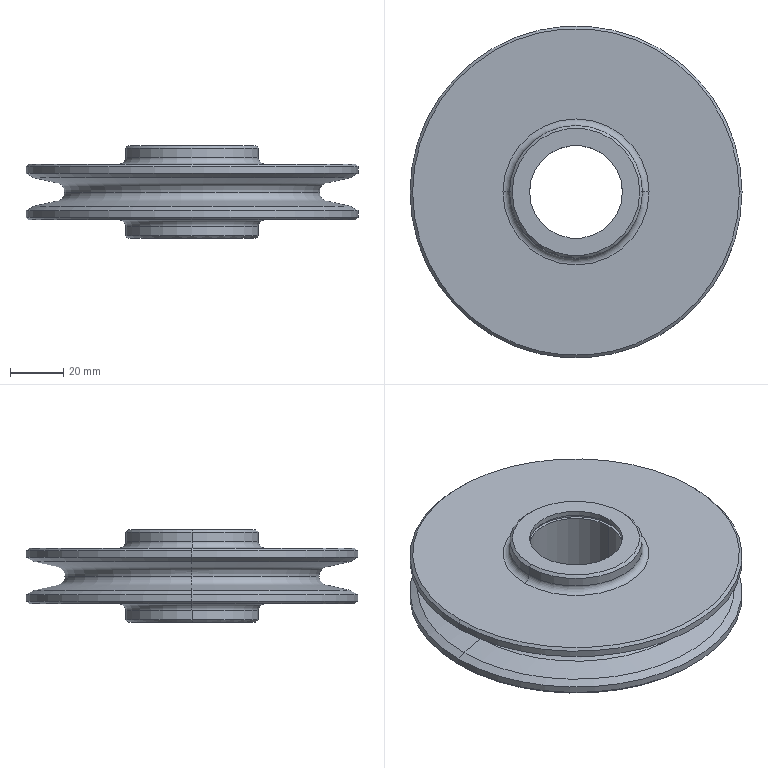Part | STEP file | POLEA IZAJE_MAMELON | 1 solid | 50 faces | box 125 x 125 x 35 mm | volume 205749 mm3 | cylinder 18 | cone 16 | torus 8 | plane 8 | commonest cylinder face diameters 35 x6 37.2 x4 50 x4 125 x4
STEP:
#1=CARTESIAN_POINT('',(-50.742,0.,-3.417));
#2=VERTEX_POINT('',#1);
#3=CARTESIAN_POINT('',(-48.,0.,0.));
#4=VERTEX_POINT('',#3);
#5=CARTESIAN_POINT('',(-51.5,0.,0.));
#6=DIRECTION('',(0.,-1.,0.));
#7=DIRECTION('',(0.,0.,-1.));
#8=AXIS2_PLACEMENT_3D('',#5,#6,#7);
#9=CIRCLE('',#8,3.5);
#10=EDGE_CURVE('',#2,#4,#9,.T.);
#11=ORIENTED_EDGE('',*,*,#10,.T.);
#12=CARTESIAN_POINT('',(48.,0.,0.));
#13=VERTEX_POINT('',#12);
#14=CARTESIAN_POINT('',(0.,0.,0.));
#15=DIRECTION('',(0.,0.,-1.));
#16=DIRECTION('',(-1.,0.,0.));
#17=AXIS2_PLACEMENT_3D('',#14,#15,#16);
#18=CIRCLE('',#17,48.);
#19=EDGE_CURVE('',#4,#13,#18,.T.);
#20=ORIENTED_EDGE('',*,*,#19,.T.);
#21=CARTESIAN_POINT('',(50.742,0.,-3.417));
#22=VERTEX_POINT('',#21);
#23=CARTESIAN_POINT('',(51.5,0.,0.));
#24=DIRECTION('',(0.,1.,0.));
#25=DIRECTION('',(-1.,0.,0.));
#26=AXIS2_PLACEMENT_3D('',#23,#24,#25);
#27=CIRCLE('',#26,3.5);
#28=EDGE_CURVE('',#22,#13,#27,.T.);
#29=ORIENTED_EDGE('',*,*,#28,.F.);
#30=CARTESIAN_POINT('',(0.,0.,-3.417));
#31=DIRECTION('',(0.,0.,-1.));
#32=DIRECTION('',(-1.,0.,0.));
#33=AXIS2_PLACEMENT_3D('',#30,#31,#32);
#34=CIRCLE('',#33,50.742);
#35=EDGE_CURVE('',#2,#22,#34,.T.);
#36=ORIENTED_EDGE('',*,*,#35,.F.);
#37=EDGE_LOOP('',(#11,#20,#29,#36));
#38=FACE_OUTER_BOUND('',#37,.T.);
#39=CARTESIAN_POINT('',(0.,0.,0.));
#40=DIRECTION('',(0.,0.,-1.));
#41=DIRECTION('',(-1.,0.,0.));
#42=AXIS2_PLACEMENT_3D('',#39,#40,#41);
#43=TOROIDAL_SURFACE('',#42,51.5,3.5);
#44=ADVANCED_FACE('',(#38),#43,.F.);
#45=ORIENTED_EDGE('',*,*,#28,.T.);
#46=CARTESIAN_POINT('',(0.,0.,0.));
#47=DIRECTION('',(0.,0.,-1.));
#48=DIRECTION('',(-1.,0.,0.));
#49=AXIS2_PLACEMENT_3D('',#46,#47,#48);
#50=CIRCLE('',#49,48.);
#51=EDGE_CURVE('',#13,#4,#50,.T.);
#52=ORIENTED_EDGE('',*,*,#51,.T.);
#53=ORIENTED_EDGE('',*,*,#10,.F.);
#54=CARTESIAN_POINT('',(0.,0.,-3.417));
#55=DIRECTION('',(0.,0.,-1.));
#56=DIRECTION('',(-1.,0.,0.));
#57=AXIS2_PLACEMENT_3D('',#54,#55,#56);
#58=CIRCLE('',#57,50.742);
#59=EDGE_CURVE('',#22,#2,#58,.T.);
#60=ORIENTED_EDGE('',*,*,#59,.F.);
#61=EDGE_LOOP('',(#45,#52,#53,#60));
#62=FACE_OUTER_BOUND('',#61,.T.);
#63=CARTESIAN_POINT('',(0.,0.,0.));
#64=DIRECTION('',(0.,0.,-1.));
#65=DIRECTION('',(-1.,0.,0.));
#66=AXIS2_PLACEMENT_3D('',#63,#64,#65);
#67=TOROIDAL_SURFACE('',#66,51.5,3.5);
#68=ADVANCED_FACE('',(#62),#67,.F.);
#69=CARTESIAN_POINT('',(61.5,0.,10.5));
#70=VERTEX_POINT('',#69);
#71=CARTESIAN_POINT('',(-61.5,0.,10.5));
#72=VERTEX_POINT('',#71);
#73=CARTESIAN_POINT('',(0.,0.,10.5));
#74=DIRECTION('',(0.,0.,1.));
#75=DIRECTION('',(-1.,0.,0.));
#76=AXIS2_PLACEMENT_3D('',#73,#74,#75);
#77=CIRCLE('',#76,61.5);
#78=EDGE_CURVE('',#70,#72,#77,.T.);
#79=ORIENTED_EDGE('',*,*,#78,.F.);
#80=CARTESIAN_POINT('',(62.5,0.,9.5));
#81=VERTEX_POINT('',#80);
#82=CARTESIAN_POINT('',(62.5,0.,9.5));
#83=DIRECTION('',(0.7071,0.,-0.7071));
#84=VECTOR('',#83,1000.);
#85=LINE('',#82,#84);
#86=EDGE_CURVE('',#70,#81,#85,.T.);
#87=ORIENTED_EDGE('',*,*,#86,.T.);
#88=CARTESIAN_POINT('',(-62.5,0.,9.5));
#89=VERTEX_POINT('',#88);
#90=CARTESIAN_POINT('',(0.,0.,9.5));
#91=DIRECTION('',(0.,0.,-1.));
#92=DIRECTION('',(-1.,0.,0.));
#93=AXIS2_PLACEMENT_3D('',#90,#91,#92);
#94=CIRCLE('',#93,62.5);
#95=EDGE_CURVE('',#89,#81,#94,.T.);
#96=ORIENTED_EDGE('',*,*,#95,.F.);
#97=CARTESIAN_POINT('',(-62.5,0.,9.5));
#98=DIRECTION('',(-0.7071,0.,-0.7071));
#99=VECTOR('',#98,1000.);
#100=LINE('',#97,#99);
#101=EDGE_CURVE('',#72,#89,#100,.T.);
#102=ORIENTED_EDGE('',*,*,#101,.F.);
#103=EDGE_LOOP('',(#79,#87,#96,#102));
#104=FACE_OUTER_BOUND('',#103,.T.);
#105=CARTESIAN_POINT('',(0.,0.,9.5));
#106=DIRECTION('',(0.,0.,-1.));
#107=DIRECTION('',(-1.,0.,0.));
#108=AXIS2_PLACEMENT_3D('',#105,#106,#107);
#109=CONICAL_SURFACE('',#108,62.5,0.7854);
#110=ADVANCED_FACE('',(#104),#109,.T.);
#111=CARTESIAN_POINT('',(-61.5,0.,-10.5));
#112=VERTEX_POINT('',#111);
#113=CARTESIAN_POINT('',(61.5,0.,-10.5));
#114=VERTEX_POINT('',#113);
#115=CARTESIAN_POINT('',(0.,0.,-10.5));
#116=DIRECTION('',(0.,0.,-1.));
#117=DIRECTION('',(1.,0.,0.));
#118=AXIS2_PLACEMENT_3D('',#115,#116,#117);
#119=CIRCLE('',#118,61.5);
#120=EDGE_CURVE('',#112,#114,#119,.T.);
#121=ORIENTED_EDGE('',*,*,#120,.F.);
#122=CARTESIAN_POINT('',(-62.5,0.,-9.5));
#123=VERTEX_POINT('',#122);
#124=CARTESIAN_POINT('',(-62.5,0.,-9.5));
#125=DIRECTION('',(-0.7071,0.,0.7071));
#126=VECTOR('',#125,1000.);
#127=LINE('',#124,#126);
#128=EDGE_CURVE('',#112,#123,#127,.T.);
#129=ORIENTED_EDGE('',*,*,#128,.T.);
#130=CARTESIAN_POINT('',(62.5,0.,-9.5));
#131=VERTEX_POINT('',#130);
#132=CARTESIAN_POINT('',(0.,0.,-9.5));
#133=DIRECTION('',(0.,0.,1.));
#134=DIRECTION('',(1.,0.,0.));
#135=AXIS2_PLACEMENT_3D('',#132,#133,#134);
#136=CIRCLE('',#135,62.5);
#137=EDGE_CURVE('',#131,#123,#136,.T.);
#138=ORIENTED_EDGE('',*,*,#137,.F.);
#139=CARTESIAN_POINT('',(62.5,0.,-9.5));
#140=DIRECTION('',(0.7071,0.,0.7071));
#141=VECTOR('',#140,1000.);
#142=LINE('',#139,#141);
#143=EDGE_CURVE('',#114,#131,#142,.T.);
#144=ORIENTED_EDGE('',*,*,#143,.F.);
#145=EDGE_LOOP('',(#121,#129,#138,#144));
#146=FACE_OUTER_BOUND('',#145,.T.);
#147=CARTESIAN_POINT('',(0.,0.,-9.5));
#148=DIRECTION('',(0.,0.,1.));
#149=DIRECTION('',(1.,0.,0.));
#150=AXIS2_PLACEMENT_3D('',#147,#148,#149);
#151=CONICAL_SURFACE('',#150,62.5,0.7854);
#152=ADVANCED_FACE('',(#146),#151,.T.);
#153=CARTESIAN_POINT('',(18.6,0.,15.6));
#154=VERTEX_POINT('',#153);
#155=CARTESIAN_POINT('',(-18.6,0.,15.6));
#156=VERTEX_POINT('',#155);
#157=CARTESIAN_POINT('',(0.,0.,15.6));
#158=DIRECTION('',(0.,0.,-1.));
#159=DIRECTION('',(-1.,0.,0.));
#160=AXIS2_PLACEMENT_3D('',#157,#158,#159);
#161=CIRCLE('',#160,18.6);
#162=EDGE_CURVE('',#154,#156,#161,.T.);
#163=ORIENTED_EDGE('',*,*,#162,.F.);
#164=CARTESIAN_POINT('',(18.6,0.,14.2));
#165=VERTEX_POINT('',#164);
#166=CARTESIAN_POINT('',(18.6,0.,-24.658));
#167=DIRECTION('',(0.,0.,-1.));
#168=VECTOR('',#167,1000.);
#169=LINE('',#166,#168);
#170=EDGE_CURVE('',#154,#165,#169,.T.);
#171=ORIENTED_EDGE('',*,*,#170,.T.);
#172=CARTESIAN_POINT('',(-18.6,0.,14.2));
#173=VERTEX_POINT('',#172);
#174=CARTESIAN_POINT('',(0.,0.,14.2));
#175=DIRECTION('',(0.,0.,-1.));
#176=DIRECTION('',(-1.,0.,0.));
#177=AXIS2_PLACEMENT_3D('',#174,#175,#176);
#178=CIRCLE('',#177,18.6);
#179=EDGE_CURVE('',#165,#173,#178,.T.);
#180=ORIENTED_EDGE('',*,*,#179,.T.);
#181=CARTESIAN_POINT('',(-18.6,0.,-24.658));
#182=DIRECTION('',(0.,0.,-1.));
#183=VECTOR('',#182,1000.);
#184=LINE('',#181,#183);
#185=EDGE_CURVE('',#156,#173,#184,.T.);
#186=ORIENTED_EDGE('',*,*,#185,.F.);
#187=EDGE_LOOP('',(#163,#171,#180,#186));
#188=FACE_OUTER_BOUND('',#187,.T.);
#189=CARTESIAN_POINT('',(0.,0.,-24.658));
#190=DIRECTION('',(0.,0.,-1.));
#191=DIRECTION('',(-1.,0.,0.));
#192=AXIS2_PLACEMENT_3D('',#189,#190,#191);
#193=CYLINDRICAL_SURFACE('',#192,18.6);
#194=ADVANCED_FACE('',(#188),#193,.F.);
#195=CARTESIAN_POINT('',(-17.5,0.,-14.2));
#196=VERTEX_POINT('',#195);
#197=CARTESIAN_POINT('',(17.5,0.,-14.2));
#198=VERTEX_POINT('',#197);
#199=CARTESIAN_POINT('',(0.,0.,-14.2));
#200=DIRECTION('',(0.,0.,1.));
#201=DIRECTION('',(-1.,0.,0.));
#202=AXIS2_PLACEMENT_3D('',#199,#200,#201);
#203=CIRCLE('',#202,17.5);
#204=EDGE_CURVE('',#196,#198,#203,.T.);
#205=ORIENTED_EDGE('',*,*,#204,.F.);
#206=CARTESIAN_POINT('',(-17.5,0.,14.2));
#207=VERTEX_POINT('',#206);
#208=CARTESIAN_POINT('',(-17.5,0.,-17.5));
#209=DIRECTION('',(0.,0.,1.));
#210=VECTOR('',#209,1000.);
#211=LINE('',#208,#210);
#212=EDGE_CURVE('',#196,#207,#211,.T.);
#213=ORIENTED_EDGE('',*,*,#212,.T.);
#214=CARTESIAN_POINT('',(17.5,0.,14.2));
#215=VERTEX_POINT('',#214);
#216=CARTESIAN_POINT('',(0.,0.,14.2));
#217=DIRECTION('',(0.,0.,-1.));
#218=DIRECTION('',(1.,0.,0.));
#219=AXIS2_PLACEMENT_3D('',#216,#217,#218);
#220=CIRCLE('',#219,17.5);
#221=EDGE_CURVE('',#215,#207,#220,.T.);
#222=ORIENTED_EDGE('',*,*,#221,.F.);
#223=CARTESIAN_POINT('',(17.5,0.,-17.5));
#224=DIRECTION('',(0.,0.,1.));
#225=VECTOR('',#224,1000.);
#226=LINE('',#223,#225);
#227=EDGE_CURVE('',#198,#215,#226,.T.);
#228=ORIENTED_EDGE('',*,*,#227,.F.);
#229=EDGE_LOOP('',(#205,#213,#222,#228));
#230=FACE_OUTER_BOUND('',#229,.T.);
#231=CARTESIAN_POINT('',(0.,0.,-17.5));
#232=DIRECTION('',(0.,0.,1.));
#233=DIRECTION('',(1.,0.,0.));
#234=AXIS2_PLACEMENT_3D('',#231,#232,#233);
#235=CYLINDRICAL_SURFACE('',#234,17.5);
#236=ADVANCED_FACE('',(#230),#235,.F.);
#237=CARTESIAN_POINT('',(18.6,0.,-14.2));
#238=VERTEX_POINT('',#237);
#239=CARTESIAN_POINT('',(-18.6,0.,-14.2));
#240=VERTEX_POINT('',#239);
#241=CARTESIAN_POINT('',(0.,0.,-14.2));
#242=DIRECTION('',(0.,0.,-1.));
#243=DIRECTION('',(-1.,0.,0.));
#244=AXIS2_PLACEMENT_3D('',#241,#242,#243);
#245=CIRCLE('',#244,18.6);
#246=EDGE_CURVE('',#238,#240,#245,.T.);
#247=ORIENTED_EDGE('',*,*,#246,.F.);
#248=CARTESIAN_POINT('',(18.6,0.,-15.6));
#249=VERTEX_POINT('',#248);
#250=CARTESIAN_POINT('',(18.6,0.,-24.658));
#251=DIRECTION('',(0.,0.,-1.));
#252=VECTOR('',#251,1000.);
#253=LINE('',#250,#252);
#254=EDGE_CURVE('',#238,#249,#253,.T.);
#255=ORIENTED_EDGE('',*,*,#254,.T.);
#256=CARTESIAN_POINT('',(-18.6,0.,-15.6));
#257=VERTEX_POINT('',#256);
#258=CARTESIAN_POINT('',(0.,0.,-15.6));
#259=DIRECTION('',(0.,0.,-1.));
#260=DIRECTION('',(-1.,0.,0.));
#261=AXIS2_PLACEMENT_3D('',#258,#259,#260);
#262=CIRCLE('',#261,18.6);
#263=EDGE_CURVE('',#249,#257,#262,.T.);
#264=ORIENTED_EDGE('',*,*,#263,.T.);
#265=CARTESIAN_POINT('',(-18.6,0.,-24.658));
#266=DIRECTION('',(0.,0.,-1.));
#267=VECTOR('',#266,1000.);
#268=LINE('',#265,#267);
#269=EDGE_CURVE('',#240,#257,#268,.T.);
#270=ORIENTED_EDGE('',*,*,#269,.F.);
#271=EDGE_LOOP('',(#247,#255,#264,#270));
#272=FACE_OUTER_BOUND('',#271,.T.);
#273=CARTESIAN_POINT('',(0.,0.,-24.658));
#274=DIRECTION('',(0.,0.,-1.));
#275=DIRECTION('',(-1.,0.,0.));
#276=AXIS2_PLACEMENT_3D('',#273,#274,#275);
#277=CYLINDRICAL_SURFACE('',#276,18.6);
#278=ADVANCED_FACE('',(#272),#277,.F.);
#279=CARTESIAN_POINT('',(24.,0.,17.5));
#280=VERTEX_POINT('',#279);
#281=CARTESIAN_POINT('',(-24.,0.,17.5));
#282=VERTEX_POINT('',#281);
#283=CARTESIAN_POINT('',(0.,0.,17.5));
#284=DIRECTION('',(0.,0.,1.));
#285=DIRECTION('',(-1.,0.,0.));
#286=AXIS2_PLACEMENT_3D('',#283,#284,#285);
#287=CIRCLE('',#286,24.);
#288=EDGE_CURVE('',#280,#282,#287,.T.);
#289=ORIENTED_EDGE('',*,*,#288,.F.);
#290=CARTESIAN_POINT('',(25.,0.,16.5));
#291=VERTEX_POINT('',#290);
#292=CARTESIAN_POINT('',(25.,0.,16.5));
#293=DIRECTION('',(0.7071,0.,-0.7071));
#294=VECTOR('',#293,1000.);
#295=LINE('',#292,#294);
#296=EDGE_CURVE('',#280,#291,#295,.T.);
#297=ORIENTED_EDGE('',*,*,#296,.T.);
#298=CARTESIAN_POINT('',(-25.,0.,16.5));
#299=VERTEX_POINT('',#298);
#300=CARTESIAN_POINT('',(0.,0.,16.5));
#301=DIRECTION('',(0.,0.,-1.));
#302=DIRECTION('',(-1.,0.,0.));
#303=AXIS2_PLACEMENT_3D('',#300,#301,#302);
#304=CIRCLE('',#303,25.);
#305=EDGE_CURVE('',#299,#291,#304,.T.);
#306=ORIENTED_EDGE('',*,*,#305,.F.);
#307=CARTESIAN_POINT('',(-25.,0.,16.5));
#308=DIRECTION('',(-0.7071,0.,-0.7071));
#309=VECTOR('',#308,1000.);
#310=LINE('',#307,#309);
#311=EDGE_CURVE('',#282,#299,#310,.T.);
#312=ORIENTED_EDGE('',*,*,#311,.F.);
#313=EDGE_LOOP('',(#289,#297,#306,#312));
#314=FACE_OUTER_BOUND('',#313,.T.);
#315=CARTESIAN_POINT('',(0.,0.,16.5));
#316=DIRECTION('',(0.,0.,-1.));
#317=DIRECTION('',(-1.,0.,0.));
#318=AXIS2_PLACEMENT_3D('',#315,#316,#317);
#319=CONICAL_SURFACE('',#318,25.,0.7854);
#320=ADVANCED_FACE('',(#314),#319,.T.);
#321=CARTESIAN_POINT('',(-24.,0.,-17.5));
#322=VERTEX_POINT('',#321);
#323=CARTESIAN_POINT('',(24.,0.,-17.5));
#324=VERTEX_POINT('',#323);
#325=CARTESIAN_POINT('',(0.,0.,-17.5));
#326=DIRECTION('',(0.,0.,-1.));
#327=DIRECTION('',(1.,0.,0.));
#328=AXIS2_PLACEMENT_3D('',#325,#326,#327);
#329=CIRCLE('',#328,24.);
#330=EDGE_CURVE('',#322,#324,#329,.T.);
#331=ORIENTED_EDGE('',*,*,#330,.F.);
#332=CARTESIAN_POINT('',(-25.,0.,-16.5));
#333=VERTEX_POINT('',#332);
#334=CARTESIAN_POINT('',(-24.,0.,-17.5));
#335=DIRECTION('',(-0.7071,0.,0.7071));
#336=VECTOR('',#335,1000.);
#337=LINE('',#334,#336);
#338=EDGE_CURVE('',#322,#333,#337,.T.);
#339=ORIENTED_EDGE('',*,*,#338,.T.);
#340=CARTESIAN_POINT('',(25.,0.,-16.5));
#341=VERTEX_POINT('',#340);
#342=CARTESIAN_POINT('',(0.,0.,-16.5));
#343=DIRECTION('',(0.,0.,1.));
#344=DIRECTION('',(1.,0.,0.));
#345=AXIS2_PLACEMENT_3D('',#342,#343,#344);
#346=CIRCLE('',#345,25.);
#347=EDGE_CURVE('',#341,#333,#346,.T.);
#348=ORIENTED_EDGE('',*,*,#347,.F.);
#349=CARTESIAN_POINT('',(24.,0.,-17.5));
#350=DIRECTION('',(0.7071,0.,0.7071));
#351=VECTOR('',#350,1000.);
#352=LINE('',#349,#351);
#353=EDGE_CURVE('',#324,#341,#352,.T.);
#354=ORIENTED_EDGE('',*,*,#353,.F.);
#355=EDGE_LOOP('',(#331,#339,#348,#354));
#356=FACE_OUTER_BOUND('',#355,.T.);
#357=CARTESIAN_POINT('',(0.,0.,-17.5));
#358=DIRECTION('',(0.,0.,1.));
#359=DIRECTION('',(1.,0.,0.));
#360=AXIS2_PLACEMENT_3D('',#357,#358,#359);
#361=CONICAL_SURFACE('',#360,24.,0.7854);
#362=ADVANCED_FACE('',(#356),#361,.T.);
#363=CARTESIAN_POINT('',(-59.688,0.,5.4));
#364=VERTEX_POINT('',#363);
#365=CARTESIAN_POINT('',(59.688,0.,5.4));
#366=VERTEX_POINT('',#365);
#367=CARTESIAN_POINT('',(0.,0.,5.4));
#368=DIRECTION('',(0.,0.,-1.));
#369=DIRECTION('',(-1.,0.,0.));
#370=AXIS2_PLACEMENT_3D('',#367,#368,#369);
#371=CIRCLE('',#370,59.688);
#372=EDGE_CURVE('',#364,#366,#371,.T.);
#373=ORIENTED_EDGE('',*,*,#372,.F.);
#374=CARTESIAN_POINT('',(-62.5,0.,7.024));
#375=VERTEX_POINT('',#374);
#376=CARTESIAN_POINT('',(-59.688,0.,5.4));
#377=DIRECTION('',(-0.866,0.,0.5));
#378=VECTOR('',#377,1000.);
#379=LINE('',#376,#378);
#380=EDGE_CURVE('',#364,#375,#379,.T.);
#381=ORIENTED_EDGE('',*,*,#380,.T.);
#382=CARTESIAN_POINT('',(62.5,0.,7.024));
#383=VERTEX_POINT('',#382);
#384=CARTESIAN_POINT('',(0.,0.,7.024));
#385=DIRECTION('',(0.,0.,1.));
#386=DIRECTION('',(1.,0.,0.));
#387=AXIS2_PLACEMENT_3D('',#384,#385,#386);
#388=CIRCLE('',#387,62.5);
#389=EDGE_CURVE('',#383,#375,#388,.T.);
#390=ORIENTED_EDGE('',*,*,#389,.F.);
#391=CARTESIAN_POINT('',(59.688,0.,5.4));
#392=DIRECTION('',(0.866,0.,0.5));
#393=VECTOR('',#392,1000.);
#394=LINE('',#391,#393);
#395=EDGE_CURVE('',#366,#383,#394,.T.);
#396=ORIENTED_EDGE('',*,*,#395,.F.);
#397=EDGE_LOOP('',(#373,#381,#390,#396));
#398=FACE_OUTER_BOUND('',#397,.T.);
#399=CARTESIAN_POINT('',(0.,0.,5.4));
#400=DIRECTION('',(0.,0.,1.));
#401=DIRECTION('',(1.,0.,0.));
#402=AXIS2_PLACEMENT_3D('',#399,#400,#401);
#403=CONICAL_SURFACE('',#402,59.688,1.047);
#404=ADVANCED_FACE('',(#398),#403,.T.);
#405=CARTESIAN_POINT('',(59.688,0.,-5.4));
#406=VERTEX_POINT('',#405);
#407=CARTESIAN_POINT('',(-59.688,0.,-5.4));
#408=VERTEX_POINT('',#407);
#409=CARTESIAN_POINT('',(0.,0.,-5.4));
#410=DIRECTION('',(0.,0.,1.));
#411=DIRECTION('',(1.,0.,0.));
#412=AXIS2_PLACEMENT_3D('',#409,#410,#411);
#413=CIRCLE('',#412,59.688);
#414=EDGE_CURVE('',#406,#408,#413,.T.);
#415=ORIENTED_EDGE('',*,*,#414,.F.);
#416=CARTESIAN_POINT('',(62.5,0.,-7.024));
#417=VERTEX_POINT('',#416);
#418=CARTESIAN_POINT('',(62.5,0.,-7.024));
#419=DIRECTION('',(0.866,0.,-0.5));
#420=VECTOR('',#419,1000.);
#421=LINE('',#418,#420);
#422=EDGE_CURVE('',#406,#417,#421,.T.);
#423=ORIENTED_EDGE('',*,*,#422,.T.);
#424=CARTESIAN_POINT('',(-62.5,0.,-7.024));
#425=VERTEX_POINT('',#424);
#426=CARTESIAN_POINT('',(0.,0.,-7.024));
#427=DIRECTION('',(0.,0.,-1.));
#428=DIRECTION('',(-1.,0.,0.));
#429=AXIS2_PLACEMENT_3D('',#426,#427,#428);
#430=CIRCLE('',#429,62.5);
#431=EDGE_CURVE('',#425,#417,#430,.T.);
#432=ORIENTED_EDGE('',*,*,#431,.F.);
#433=CARTESIAN_POINT('',(-62.5,0.,-7.024));
#434=DIRECTION('',(-0.866,0.,-0.5));
#435=VECTOR('',#434,1000.);
#436=LINE('',#433,#435);
#437=EDGE_CURVE('',#408,#425,#436,.T.);
#438=ORIENTED_EDGE('',*,*,#437,.F.);
#439=EDGE_LOOP('',(#415,#423,#432,#438));
#440=FACE_OUTER_BOUND('',#439,.T.);
#441=CARTESIAN_POINT('',(0.,0.,-7.024));
#442=DIRECTION('',(0.,0.,-1.));
#443=DIRECTION('',(-1.,0.,0.));
#444=AXIS2_PLACEMENT_3D('',#441,#442,#443);
#445=CONICAL_SURFACE('',#444,62.5,1.047);
#446=ADVANCED_FACE('',(#440),#445,.T.);
#447=CARTESIAN_POINT('',(27.5,0.,10.5));
#448=VERTEX_POINT('',#447);
#449=CARTESIAN_POINT('',(-27.5,0.,10.5));
#450=VERTEX_POINT('',#449);
#451=CARTESIAN_POINT('',(0.,0.,10.5));
#452=DIRECTION('',(0.,0.,-1.));
#453=DIRECTION('',(-1.,0.,0.));
#454=AXIS2_PLACEMENT_3D('',#451,#452,#453);
#455=CIRCLE('',#454,27.5);
#456=EDGE_CURVE('',#448,#450,#455,.T.);
#457=ORIENTED_EDGE('',*,*,#456,.F.);
#458=CARTESIAN_POINT('',(25.,0.,13.));
#459=VERTEX_POINT('',#458);
#460=CARTESIAN_POINT('',(27.5,0.,13.));
#461=DIRECTION('',(0.,1.,0.));
#462=DIRECTION('',(-1.,0.,0.));
#463=AXIS2_PLACEMENT_3D('',#460,#461,#462);
#464=CIRCLE('',#463,2.5);
#465=EDGE_CURVE('',#448,#459,#464,.T.);
#466=ORIENTED_EDGE('',*,*,#465,.T.);
#467=CARTESIAN_POINT('',(-25.,0.,13.));
#468=VERTEX_POINT('',#467);
#469=CARTESIAN_POINT('',(0.,0.,13.));
#470=DIRECTION('',(0.,0.,1.));
#471=DIRECTION('',(-1.,0.,0.));
#472=AXIS2_PLACEMENT_3D('',#469,#470,#471);
#473=CIRCLE('',#472,25.);
#474=EDGE_CURVE('',#468,#459,#473,.T.);
#475=ORIENTED_EDGE('',*,*,#474,.F.);
#476=CARTESIAN_POINT('',(-27.5,0.,13.));
#477=DIRECTION('',(0.,-1.,0.));
#478=DIRECTION('',(0.,0.,-1.));
#479=AXIS2_PLACEMENT_3D('',#476,#477,#478);
#480=CIRCLE('',#479,2.5);
#481=EDGE_CURVE('',#450,#468,#480,.T.);
#482=ORIENTED_EDGE('',*,*,#481,.F.);
#483=EDGE_LOOP('',(#457,#466,#475,#482));
#484=FACE_OUTER_BOUND('',#483,.T.);
#485=CARTESIAN_POINT('',(0.,0.,13.));
#486=DIRECTION('',(0.,0.,-1.));
#487=DIRECTION('',(-1.,0.,0.));
#488=AXIS2_PLACEMENT_3D('',#485,#486,#487);
#489=TOROIDAL_SURFACE('',#488,27.5,2.5);
#490=ADVANCED_FACE('',(#484),#489,.F.);
#491=CARTESIAN_POINT('',(-27.5,0.,-10.5));
#492=VERTEX_POINT('',#491);
#493=CARTESIAN_POINT('',(27.5,0.,-10.5));
#494=VERTEX_POINT('',#493);
#495=CARTESIAN_POINT('',(0.,0.,-10.5));
#496=DIRECTION('',(0.,0.,1.));
#497=DIRECTION('',(1.,0.,0.));
#498=AXIS2_PLACEMENT_3D('',#495,#496,#497);
#499=CIRCLE('',#498,27.5);
#500=EDGE_CURVE('',#492,#494,#499,.T.);
#501=ORIENTED_EDGE('',*,*,#500,.F.);
#502=CARTESIAN_POINT('',(-25.,0.,-13.));
#503=VERTEX_POINT('',#502);
#504=CARTESIAN_POINT('',(-27.5,0.,-13.));
#505=DIRECTION('',(0.,1.,0.));
#506=DIRECTION('',(-1.,0.,0.));
#507=AXIS2_PLACEMENT_3D('',#504,#505,#506);
#508=CIRCLE('',#507,2.5);
#509=EDGE_CURVE('',#492,#503,#508,.T.);
#510=ORIENTED_EDGE('',*,*,#509,.T.);
#511=CARTESIAN_POINT('',(25.,0.,-13.));
#512=VERTEX_POINT('',#511);
#513=CARTESIAN_POINT('',(0.,0.,-13.));
#514=DIRECTION('',(0.,0.,-1.));
#515=DIRECTION('',(1.,0.,0.));
#516=AXIS2_PLACEMENT_3D('',#513,#514,#515);
#517=CIRCLE('',#516,25.);
#518=EDGE_CURVE('',#512,#503,#517,.T.);
#519=ORIENTED_EDGE('',*,*,#518,.F.);
#520=CARTESIAN_POINT('',(27.5,0.,-13.));
#521=DIRECTION('',(0.,-1.,0.));
#522=DIRECTION('',(0.,0.,-1.));
#523=AXIS2_PLACEMENT_3D('',#520,#521,#522);
#524=CIRCLE('',#523,2.5);
#525=EDGE_CURVE('',#494,#512,#524,.T.);
#526=ORIENTED_EDGE('',*,*,#525,.F.);
#527=EDGE_LOOP('',(#501,#510,#519,#526));
#528=FACE_OUTER_BOUND('',#527,.T.);
#529=CARTESIAN_POINT('',(0.,0.,-13.));
#530=DIRECTION('',(0.,0.,1.));
#531=DIRECTION('',(1.,0.,0.));
#532=AXIS2_PLACEMENT_3D('',#529,#530,#531);
#533=TOROIDAL_SURFACE('',#532,27.5,2.5);
#534=ADVANCED_FACE('',(#528),#533,.F.);
#535=ORIENTED_EDGE('',*,*,#305,.T.);
#536=CARTESIAN_POINT('',(25.,0.,-31.613));
#537=DIRECTION('',(0.,0.,-1.));
#538=VECTOR('',#537,1000.);
#539=LINE('',#536,#538);
#540=EDGE_CURVE('',#291,#459,#539,.T.);
#541=ORIENTED_EDGE('',*,*,#540,.T.);
#542=CARTESIAN_POINT('',(0.,0.,13.));
#543=DIRECTION('',(0.,0.,1.));
#544=DIRECTION('',(-1.,0.,0.));
#545=AXIS2_PLACEMENT_3D('',#542,#543,#544);
#546=CIRCLE('',#545,25.);
#547=EDGE_CURVE('',#459,#468,#546,.T.);
#548=ORIENTED_EDGE('',*,*,#547,.T.);
#549=CARTESIAN_POINT('',(-25.,0.,-31.613));
#550=DIRECTION('',(0.,0.,-1.));
#551=VECTOR('',#550,1000.);
#552=LINE('',#549,#551);
#553=EDGE_CURVE('',#299,#468,#552,.T.);
#554=ORIENTED_EDGE('',*,*,#553,.F.);
#555=EDGE_LOOP('',(#535,#541,#548,#554));
#556=FACE_OUTER_BOUND('',#555,.T.);
#557=CARTESIAN_POINT('',(0.,0.,-31.613));
#558=DIRECTION('',(0.,0.,-1.));
#559=DIRECTION('',(-1.,0.,0.));
#560=AXIS2_PLACEMENT_3D('',#557,#558,#559);
#561=CYLINDRICAL_SURFACE('',#560,25.);
#562=ADVANCED_FACE('',(#556),#561,.T.);
#563=CARTESIAN_POINT('',(0.,0.,-13.));
#564=DIRECTION('',(0.,0.,-1.));
#565=DIRECTION('',(1.,0.,0.));
#566=AXIS2_PLACEMENT_3D('',#563,#564,#565);
#567=CIRCLE('',#566,25.);
#568=EDGE_CURVE('',#503,#512,#567,.T.);
#569=ORIENTED_EDGE('',*,*,#568,.T.);
#570=CARTESIAN_POINT('',(25.,0.,-31.613));
#571=DIRECTION('',(0.,0.,-1.));
#572=VECTOR('',#571,1000.);
#573=LINE('',#570,#572);
#574=EDGE_CURVE('',#512,#341,#573,.T.);
#575=ORIENTED_EDGE('',*,*,#574,.T.);
#576=ORIENTED_EDGE('',*,*,#347,.T.);
#577=CARTESIAN_POINT('',(-25.,0.,-31.613));
#578=DIRECTION('',(0.,0.,-1.));
#579=VECTOR('',#578,1000.);
#580=LINE('',#577,#579);
#581=EDGE_CURVE('',#503,#333,#580,.T.);
#582=ORIENTED_EDGE('',*,*,#581,.F.);
#583=EDGE_LOOP('',(#569,#575,#576,#582));
#584=FACE_OUTER_BOUND('',#583,.T.);
#585=CARTESIAN_POINT('',(0.,0.,-31.613));
#586=DIRECTION('',(0.,0.,-1.));
#587=DIRECTION('',(-1.,0.,0.));
#588=AXIS2_PLACEMENT_3D('',#585,#586,#587);
#589=CYLINDRICAL_SURFACE('',#588,25.);
#590=ADVANCED_FACE('',(#584),#589,.T.);
#591=ORIENTED_EDGE('',*,*,#137,.T.);
#592=CARTESIAN_POINT('',(-62.5,0.,17.5));
#593=DIRECTION('',(0.,0.,1.));
#594=VECTOR('',#593,1000.);
#595=LINE('',#592,#594);
#596=EDGE_CURVE('',#123,#425,#595,.T.);
#597=ORIENTED_EDGE('',*,*,#596,.T.);
#598=ORIENTED_EDGE('',*,*,#431,.T.);
#599=CARTESIAN_POINT('',(62.5,0.,17.5));
#600=DIRECTION('',(0.,0.,1.));
#601=VECTOR('',#600,1000.);
#602=LINE('',#599,#601);
#603=EDGE_CURVE('',#131,#417,#602,.T.);
#604=ORIENTED_EDGE('',*,*,#603,.F.);
#605=EDGE_LOOP('',(#591,#597,#598,#604));
#606=FACE_OUTER_BOUND('',#605,.T.);
#607=CARTESIAN_POINT('',(0.,0.,17.5));
#608=DIRECTION('',(0.,0.,1.));
#609=DIRECTION('',(1.,0.,0.));
#610=AXIS2_PLACEMENT_3D('',#607,#608,#609);
#611=CYLINDRICAL_SURFACE('',#610,62.5);
#612=ADVANCED_FACE('',(#606),#611,.T.);
#613=ORIENTED_EDGE('',*,*,#35,.T.);
#614=CARTESIAN_POINT('',(50.742,0.,-3.417));
#615=DIRECTION('',(0.9763,0.,-0.2164));
#616=VECTOR('',#615,1000.);
#617=LINE('',#614,#616);
#618=EDGE_CURVE('',#22,#406,#617,.T.);
#619=ORIENTED_EDGE('',*,*,#618,.T.);
#620=ORIENTED_EDGE('',*,*,#414,.T.);
#621=CARTESIAN_POINT('',(-50.742,0.,-3.417));
#622=DIRECTION('',(-0.9763,0.,-0.2164));
#623=VECTOR('',#622,1000.);
#624=LINE('',#621,#623);
#625=EDGE_CURVE('',#2,#408,#624,.T.);
#626=ORIENTED_EDGE('',*,*,#625,.F.);
#627=EDGE_LOOP('',(#613,#619,#620,#626));
#628=FACE_OUTER_BOUND('',#627,.T.);
#629=CARTESIAN_POINT('',(0.,0.,-3.417));
#630=DIRECTION('',(0.,0.,-1.));
#631=DIRECTION('',(-1.,0.,0.));
#632=AXIS2_PLACEMENT_3D('',#629,#630,#631);
#633=CONICAL_SURFACE('',#632,50.742,1.353);
#634=ADVANCED_FACE('',(#628),#633,.T.);
#635=ORIENTED_EDGE('',*,*,#51,.F.);
#636=CARTESIAN_POINT('',(50.742,0.,3.417));
#637=VERTEX_POINT('',#636);
#638=CARTESIAN_POINT('',(51.5,0.,0.));
#639=DIRECTION('',(0.,1.,0.));
#640=DIRECTION('',(-1.,0.,0.));
#641=AXIS2_PLACEMENT_3D('',#638,#639,#640);
#642=CIRCLE('',#641,3.5);
#643=EDGE_CURVE('',#13,#637,#642,.T.);
#644=ORIENTED_EDGE('',*,*,#643,.T.);
#645=CARTESIAN_POINT('',(-50.742,0.,3.417));
#646=VERTEX_POINT('',#645);
#647=CARTESIAN_POINT('',(0.,0.,3.417));
#648=DIRECTION('',(0.,0.,-1.));
#649=DIRECTION('',(-1.,0.,0.));
#650=AXIS2_PLACEMENT_3D('',#647,#648,#649);
#651=CIRCLE('',#650,50.742);
#652=EDGE_CURVE('',#637,#646,#651,.T.);
#653=ORIENTED_EDGE('',*,*,#652,.T.);
#654=CARTESIAN_POINT('',(-51.5,0.,0.));
#655=DIRECTION('',(0.,-1.,0.));
#656=DIRECTION('',(0.,0.,-1.));
#657=AXIS2_PLACEMENT_3D('',#654,#655,#656);
#658=CIRCLE('',#657,3.5);
#659=EDGE_CURVE('',#4,#646,#658,.T.);
#660=ORIENTED_EDGE('',*,*,#659,.F.);
#661=EDGE_LOOP('',(#635,#644,#653,#660));
#662=FACE_OUTER_BOUND('',#661,.T.);
#663=CARTESIAN_POINT('',(0.,0.,0.));
#664=DIRECTION('',(0.,0.,-1.));
#665=DIRECTION('',(-1.,0.,0.));
#666=AXIS2_PLACEMENT_3D('',#663,#664,#665);
#667=TOROIDAL_SURFACE('',#666,51.5,3.5);
#668=ADVANCED_FACE('',(#662),#667,.F.);
#669=CARTESIAN_POINT('',(0.,0.,3.417));
#670=DIRECTION('',(0.,0.,-1.));
#671=DIRECTION('',(-1.,0.,0.));
#672=AXIS2_PLACEMENT_3D('',#669,#670,#671);
#673=CIRCLE('',#672,50.742);
#674=EDGE_CURVE('',#646,#637,#673,.T.);
#675=ORIENTED_EDGE('',*,*,#674,.F.);
#676=CARTESIAN_POINT('',(-62.5,0.,6.024));
#677=DIRECTION('',(-0.9763,0.,0.2164));
#678=VECTOR('',#677,1000.);
#679=LINE('',#676,#678);
#680=EDGE_CURVE('',#646,#364,#679,.T.);
#681=ORIENTED_EDGE('',*,*,#680,.T.);
#682=ORIENTED_EDGE('',*,*,#372,.T.);
#683=CARTESIAN_POINT('',(62.5,0.,6.024));
#684=DIRECTION('',(0.9763,0.,0.2164));
#685=VECTOR('',#684,1000.);
#686=LINE('',#683,#685);
#687=EDGE_CURVE('',#637,#366,#686,.T.);
#688=ORIENTED_EDGE('',*,*,#687,.F.);
#689=EDGE_LOOP('',(#675,#681,#682,#688));
#690=FACE_OUTER_BOUND('',#689,.T.);
#691=CARTESIAN_POINT('',(0.,0.,6.024));
#692=DIRECTION('',(0.,0.,1.));
#693=DIRECTION('',(1.,0.,0.));
#694=AXIS2_PLACEMENT_3D('',#691,#692,#693);
#695=CONICAL_SURFACE('',#694,62.5,1.353);
#696=ADVANCED_FACE('',(#690),#695,.T.);
#697=ORIENTED_EDGE('',*,*,#389,.T.);
#698=CARTESIAN_POINT('',(-62.5,0.,17.5));
#699=DIRECTION('',(0.,0.,1.));
#700=VECTOR('',#699,1000.);
#701=LINE('',#698,#700);
#702=EDGE_CURVE('',#375,#89,#701,.T.);
#703=ORIENTED_EDGE('',*,*,#702,.T.);
#704=ORIENTED_EDGE('',*,*,#95,.T.);
#705=CARTESIAN_POINT('',(62.5,0.,17.5));
#706=DIRECTION('',(0.,0.,1.));
#707=VECTOR('',#706,1000.);
#708=LINE('',#705,#707);
#709=EDGE_CURVE('',#383,#81,#708,.T.);
#710=ORIENTED_EDGE('',*,*,#709,.F.);
#711=EDGE_LOOP('',(#697,#703,#704,#710));
#712=FACE_OUTER_BOUND('',#711,.T.);
#713=CARTESIAN_POINT('',(0.,0.,17.5));
#714=DIRECTION('',(0.,0.,1.));
#715=DIRECTION('',(1.,0.,0.));
#716=AXIS2_PLACEMENT_3D('',#713,#714,#715);
#717=CYLINDRICAL_SURFACE('',#716,62.5);
#718=ADVANCED_FACE('',(#712),#717,.T.);
#719=CARTESIAN_POINT('',(-17.5,0.,-17.5));
#720=VERTEX_POINT('',#719);
#721=CARTESIAN_POINT('',(17.5,0.,-17.5));
#722=VERTEX_POINT('',#721);
#723=CARTESIAN_POINT('',(0.,0.,-17.5));
#724=DIRECTION('',(0.,0.,1.));
#725=DIRECTION('',(1.,0.,0.));
#726=AXIS2_PLACEMENT_3D('',#723,#724,#725);
#727=CIRCLE('',#726,17.5);
#728=EDGE_CURVE('',#720,#722,#727,.T.);
#729=ORIENTED_EDGE('',*,*,#728,.F.);
#730=CARTESIAN_POINT('',(-17.5,0.,-15.6));
#731=VERTEX_POINT('',#730);
#732=CARTESIAN_POINT('',(-17.5,0.,-17.5));
#733=DIRECTION('',(0.,0.,1.));
#734=VECTOR('',#733,1000.);
#735=LINE('',#732,#734);
#736=EDGE_CURVE('',#720,#731,#735,.T.);
#737=ORIENTED_EDGE('',*,*,#736,.T.);
#738=CARTESIAN_POINT('',(17.5,0.,-15.6));
#739=VERTEX_POINT('',#738);
#740=CARTESIAN_POINT('',(0.,0.,-15.6));
#741=DIRECTION('',(0.,0.,-1.));
#742=DIRECTION('',(1.,0.,0.));
#743=AXIS2_PLACEMENT_3D('',#740,#741,#742);
#744=CIRCLE('',#743,17.5);
#745=EDGE_CURVE('',#739,#731,#744,.T.);
#746=ORIENTED_EDGE('',*,*,#745,.F.);
#747=CARTESIAN_POINT('',(17.5,0.,-17.5));
#748=DIRECTION('',(0.,0.,1.));
#749=VECTOR('',#748,1000.);
#750=LINE('',#747,#749);
#751=EDGE_CURVE('',#722,#739,#750,.T.);
#752=ORIENTED_EDGE('',*,*,#751,.F.);
#753=EDGE_LOOP('',(#729,#737,#746,#752));
#754=FACE_OUTER_BOUND('',#753,.T.);
#755=CARTESIAN_POINT('',(0.,0.,-17.5));
#756=DIRECTION('',(0.,0.,1.));
#757=DIRECTION('',(1.,0.,0.));
#758=AXIS2_PLACEMENT_3D('',#755,#756,#757);
#759=CYLINDRICAL_SURFACE('',#758,17.5);
#760=ADVANCED_FACE('',(#754),#759,.F.);
#761=CARTESIAN_POINT('',(-17.5,0.,15.6));
#762=VERTEX_POINT('',#761);
#763=CARTESIAN_POINT('',(17.5,0.,15.6));
#764=VERTEX_POINT('',#763);
#765=CARTESIAN_POINT('',(0.,0.,15.6));
#766=DIRECTION('',(0.,0.,1.));
#767=DIRECTION('',(-1.,0.,0.));
#768=AXIS2_PLACEMENT_3D('',#765,#766,#767);
#769=CIRCLE('',#768,17.5);
#770=EDGE_CURVE('',#762,#764,#769,.T.);
#771=ORIENTED_EDGE('',*,*,#770,.F.);
#772=CARTESIAN_POINT('',(-17.5,0.,17.5));
#773=VERTEX_POINT('',#772);
#774=CARTESIAN_POINT('',(-17.5,0.,-17.5));
#775=DIRECTION('',(0.,0.,1.));
#776=VECTOR('',#775,1000.);
#777=LINE('',#774,#776);
#778=EDGE_CURVE('',#762,#773,#777,.T.);
#779=ORIENTED_EDGE('',*,*,#778,.T.);
#780=CARTESIAN_POINT('',(17.5,0.,17.5));
#781=VERTEX_POINT('',#780);
#782=CARTESIAN_POINT('',(0.,0.,17.5));
#783=DIRECTION('',(0.,0.,1.));
#784=DIRECTION('',(1.,0.,0.));
#785=AXIS2_PLACEMENT_3D('',#782,#783,#784);
#786=CIRCLE('',#785,17.5);
#787=EDGE_CURVE('',#773,#781,#786,.T.);
#788=ORIENTED_EDGE('',*,*,#787,.T.);
#789=CARTESIAN_POINT('',(17.5,0.,-17.5));
#790=DIRECTION('',(0.,0.,1.));
#791=VECTOR('',#790,1000.);
#792=LINE('',#789,#791);
#793=EDGE_CURVE('',#764,#781,#792,.T.);
#794=ORIENTED_EDGE('',*,*,#793,.F.);
#795=EDGE_LOOP('',(#771,#779,#788,#794));
#796=FACE_OUTER_BOUND('',#795,.T.);
#797=CARTESIAN_POINT('',(0.,0.,-17.5));
#798=DIRECTION('',(0.,0.,1.));
#799=DIRECTION('',(1.,0.,0.));
#800=AXIS2_PLACEMENT_3D('',#797,#798,#799);
#801=CYLINDRICAL_SURFACE('',#800,17.5);
#802=ADVANCED_FACE('',(#796),#801,.F.);
#803=ORIENTED_EDGE('',*,*,#778,.F.);
#804=CARTESIAN_POINT('',(0.,0.,15.6));
#805=DIRECTION('',(0.,0.,1.));
#806=DIRECTION('',(-1.,0.,0.));
#807=AXIS2_PLACEMENT_3D('',#804,#805,#806);
#808=CIRCLE('',#807,17.5);
#809=EDGE_CURVE('',#764,#762,#808,.T.);
#810=ORIENTED_EDGE('',*,*,#809,.F.);
#811=ORIENTED_EDGE('',*,*,#793,.T.);
#812=CARTESIAN_POINT('',(0.,0.,17.5));
#813=DIRECTION('',(0.,0.,1.));
#814=DIRECTION('',(1.,0.,0.));
#815=AXIS2_PLACEMENT_3D('',#812,#813,#814);
#816=CIRCLE('',#815,17.5);
#817=EDGE_CURVE('',#781,#773,#816,.T.);
#818=ORIENTED_EDGE('',*,*,#817,.T.);
#819=EDGE_LOOP('',(#803,#810,#811,#818));
#820=FACE_OUTER_BOUND('',#819,.T.);
#821=CARTESIAN_POINT('',(0.,0.,-17.5));
#822=DIRECTION('',(0.,0.,1.));
#823=DIRECTION('',(1.,0.,0.));
#824=AXIS2_PLACEMENT_3D('',#821,#822,#823);
#825=CYLINDRICAL_SURFACE('',#824,17.5);
#826=ADVANCED_FACE('',(#820),#825,.F.);
#827=ORIENTED_EDGE('',*,*,#736,.F.);
#828=CARTESIAN_POINT('',(0.,0.,-17.5));
#829=DIRECTION('',(0.,0.,1.));
#830=DIRECTION('',(1.,0.,0.));
#831=AXIS2_PLACEMENT_3D('',#828,#829,#830);
#832=CIRCLE('',#831,17.5);
#833=EDGE_CURVE('',#722,#720,#832,.T.);
#834=ORIENTED_EDGE('',*,*,#833,.F.);
#835=ORIENTED_EDGE('',*,*,#751,.T.);
#836=CARTESIAN_POINT('',(0.,0.,-15.6));
#837=DIRECTION('',(0.,0.,-1.));
#838=DIRECTION('',(1.,0.,0.));
#839=AXIS2_PLACEMENT_3D('',#836,#837,#838);
#840=CIRCLE('',#839,17.5);
#841=EDGE_CURVE('',#731,#739,#840,.T.);
#842=ORIENTED_EDGE('',*,*,#841,.F.);
#843=EDGE_LOOP('',(#827,#834,#835,#842));
#844=FACE_OUTER_BOUND('',#843,.T.);
#845=CARTESIAN_POINT('',(0.,0.,-17.5));
#846=DIRECTION('',(0.,0.,1.));
#847=DIRECTION('',(1.,0.,0.));
#848=AXIS2_PLACEMENT_3D('',#845,#846,#847);
#849=CYLINDRICAL_SURFACE('',#848,17.5);
#850=ADVANCED_FACE('',(#844),#849,.F.);
#851=ORIENTED_EDGE('',*,*,#702,.F.);
#852=CARTESIAN_POINT('',(0.,0.,7.024));
#853=DIRECTION('',(0.,0.,1.));
#854=DIRECTION('',(1.,0.,0.));
#855=AXIS2_PLACEMENT_3D('',#852,#853,#854);
#856=CIRCLE('',#855,62.5);
#857=EDGE_CURVE('',#375,#383,#856,.T.);
#858=ORIENTED_EDGE('',*,*,#857,.T.);
#859=ORIENTED_EDGE('',*,*,#709,.T.);
#860=CARTESIAN_POINT('',(0.,0.,9.5));
#861=DIRECTION('',(0.,0.,-1.));
#862=DIRECTION('',(-1.,0.,0.));
#863=AXIS2_PLACEMENT_3D('',#860,#861,#862);
#864=CIRCLE('',#863,62.5);
#865=EDGE_CURVE('',#81,#89,#864,.T.);
#866=ORIENTED_EDGE('',*,*,#865,.T.);
#867=EDGE_LOOP('',(#851,#858,#859,#866));
#868=FACE_OUTER_BOUND('',#867,.T.);
#869=CARTESIAN_POINT('',(0.,0.,17.5));
#870=DIRECTION('',(0.,0.,1.));
#871=DIRECTION('',(1.,0.,0.));
#872=AXIS2_PLACEMENT_3D('',#869,#870,#871);
#873=CYLINDRICAL_SURFACE('',#872,62.5);
#874=ADVANCED_FACE('',(#868),#873,.T.);
#875=ORIENTED_EDGE('',*,*,#680,.F.);
#876=ORIENTED_EDGE('',*,*,#652,.F.);
#877=ORIENTED_EDGE('',*,*,#687,.T.);
#878=CARTESIAN_POINT('',(0.,0.,5.4));
#879=DIRECTION('',(0.,0.,-1.));
#880=DIRECTION('',(-1.,0.,0.));
#881=AXIS2_PLACEMENT_3D('',#878,#879,#880);
#882=CIRCLE('',#881,59.688);
#883=EDGE_CURVE('',#366,#364,#882,.T.);
#884=ORIENTED_EDGE('',*,*,#883,.T.);
#885=EDGE_LOOP('',(#875,#876,#877,#884));
#886=FACE_OUTER_BOUND('',#885,.T.);
#887=CARTESIAN_POINT('',(0.,0.,6.024));
#888=DIRECTION('',(0.,0.,1.));
#889=DIRECTION('',(1.,0.,0.));
#890=AXIS2_PLACEMENT_3D('',#887,#888,#889);
#891=CONICAL_SURFACE('',#890,62.5,1.353);
#892=ADVANCED_FACE('',(#886),#891,.T.);
#893=ORIENTED_EDGE('',*,*,#19,.F.);
#894=ORIENTED_EDGE('',*,*,#659,.T.);
#895=ORIENTED_EDGE('',*,*,#674,.T.);
#896=ORIENTED_EDGE('',*,*,#643,.F.);
#897=EDGE_LOOP('',(#893,#894,#895,#896));
#898=FACE_OUTER_BOUND('',#897,.T.);
#899=CARTESIAN_POINT('',(0.,0.,0.));
#900=DIRECTION('',(0.,0.,-1.));
#901=DIRECTION('',(-1.,0.,0.));
#902=AXIS2_PLACEMENT_3D('',#899,#900,#901);
#903=TOROIDAL_SURFACE('',#902,51.5,3.5);
#904=ADVANCED_FACE('',(#898),#903,.F.);
#905=ORIENTED_EDGE('',*,*,#618,.F.);
#906=ORIENTED_EDGE('',*,*,#59,.T.);
#907=ORIENTED_EDGE('',*,*,#625,.T.);
#908=CARTESIAN_POINT('',(0.,0.,-5.4));
#909=DIRECTION('',(0.,0.,1.));
#910=DIRECTION('',(1.,0.,0.));
#911=AXIS2_PLACEMENT_3D('',#908,#909,#910);
#912=CIRCLE('',#911,59.688);
#913=EDGE_CURVE('',#408,#406,#912,.T.);
#914=ORIENTED_EDGE('',*,*,#913,.T.);
#915=EDGE_LOOP('',(#905,#906,#907,#914));
#916=FACE_OUTER_BOUND('',#915,.T.);
#917=CARTESIAN_POINT('',(0.,0.,-3.417));
#918=DIRECTION('',(0.,0.,-1.));
#919=DIRECTION('',(-1.,0.,0.));
#920=AXIS2_PLACEMENT_3D('',#917,#918,#919);
#921=CONICAL_SURFACE('',#920,50.742,1.353);
#922=ADVANCED_FACE('',(#916),#921,.T.);
#923=ORIENTED_EDGE('',*,*,#596,.F.);
#924=CARTESIAN_POINT('',(0.,0.,-9.5));
#925=DIRECTION('',(0.,0.,1.));
#926=DIRECTION('',(1.,0.,0.));
#927=AXIS2_PLACEMENT_3D('',#924,#925,#926);
#928=CIRCLE('',#927,62.5);
#929=EDGE_CURVE('',#123,#131,#928,.T.);
#930=ORIENTED_EDGE('',*,*,#929,.T.);
#931=ORIENTED_EDGE('',*,*,#603,.T.);
#932=CARTESIAN_POINT('',(0.,0.,-7.024));
#933=DIRECTION('',(0.,0.,-1.));
#934=DIRECTION('',(-1.,0.,0.));
#935=AXIS2_PLACEMENT_3D('',#932,#933,#934);
#936=CIRCLE('',#935,62.5);
#937=EDGE_CURVE('',#417,#425,#936,.T.);
#938=ORIENTED_EDGE('',*,*,#937,.T.);
#939=EDGE_LOOP('',(#923,#930,#931,#938));
#940=FACE_OUTER_BOUND('',#939,.T.);
#941=CARTESIAN_POINT('',(0.,0.,17.5));
#942=DIRECTION('',(0.,0.,1.));
#943=DIRECTION('',(1.,0.,0.));
#944=AXIS2_PLACEMENT_3D('',#941,#942,#943);
#945=CYLINDRICAL_SURFACE('',#944,62.5);
#946=ADVANCED_FACE('',(#940),#945,.T.);
#947=CARTESIAN_POINT('',(0.,0.,-10.5));
#948=DIRECTION('',(0.,0.,-1.));
#949=DIRECTION('',(1.,0.,0.));
#950=AXIS2_PLACEMENT_3D('',#947,#948,#949);
#951=CIRCLE('',#950,61.5);
#952=EDGE_CURVE('',#114,#112,#951,.T.);
#953=ORIENTED_EDGE('',*,*,#952,.T.);
#954=ORIENTED_EDGE('',*,*,#120,.T.);
#955=EDGE_LOOP('',(#953,#954));
#956=FACE_OUTER_BOUND('',#955,.T.);
#957=CARTESIAN_POINT('',(0.,0.,-10.5));
#958=DIRECTION('',(0.,0.,1.));
#959=DIRECTION('',(1.,0.,0.));
#960=AXIS2_PLACEMENT_3D('',#957,#958,#959);
#961=CIRCLE('',#960,27.5);
#962=EDGE_CURVE('',#494,#492,#961,.T.);
#963=ORIENTED_EDGE('',*,*,#962,.T.);
#964=ORIENTED_EDGE('',*,*,#500,.T.);
#965=EDGE_LOOP('',(#963,#964));
#966=FACE_BOUND('',#965,.T.);
#967=CARTESIAN_POINT('',(0.,65.922,-10.5));
#968=DIRECTION('',(0.,0.,1.));
#969=DIRECTION('',(1.,0.,0.));
#970=AXIS2_PLACEMENT_3D('',#967,#968,#969);
#971=PLANE('',#970);
#972=ADVANCED_FACE('',(#956,#966),#971,.F.);
#973=ORIENTED_EDGE('',*,*,#574,.F.);
#974=ORIENTED_EDGE('',*,*,#518,.T.);
#975=ORIENTED_EDGE('',*,*,#581,.T.);
#976=CARTESIAN_POINT('',(0.,0.,-16.5));
#977=DIRECTION('',(0.,0.,1.));
#978=DIRECTION('',(1.,0.,0.));
#979=AXIS2_PLACEMENT_3D('',#976,#977,#978);
#980=CIRCLE('',#979,25.);
#981=EDGE_CURVE('',#333,#341,#980,.T.);
#982=ORIENTED_EDGE('',*,*,#981,.T.);
#983=EDGE_LOOP('',(#973,#974,#975,#982));
#984=FACE_OUTER_BOUND('',#983,.T.);
#985=CARTESIAN_POINT('',(0.,0.,-31.613));
#986=DIRECTION('',(0.,0.,-1.));
#987=DIRECTION('',(-1.,0.,0.));
#988=AXIS2_PLACEMENT_3D('',#985,#986,#987);
#989=CYLINDRICAL_SURFACE('',#988,25.);
#990=ADVANCED_FACE('',(#984),#989,.T.);
#991=CARTESIAN_POINT('',(0.,0.,17.5));
#992=DIRECTION('',(0.,0.,1.));
#993=DIRECTION('',(-1.,0.,0.));
#994=AXIS2_PLACEMENT_3D('',#991,#992,#993);
#995=CIRCLE('',#994,24.);
#996=EDGE_CURVE('',#282,#280,#995,.T.);
#997=ORIENTED_EDGE('',*,*,#996,.T.);
#998=ORIENTED_EDGE('',*,*,#288,.T.);
#999=EDGE_LOOP('',(#997,#998));
#1000=FACE_OUTER_BOUND('',#999,.T.);
#1001=ORIENTED_EDGE('',*,*,#817,.F.);
#1002=ORIENTED_EDGE('',*,*,#787,.F.);
#1003=EDGE_LOOP('',(#1001,#1002));
#1004=FACE_BOUND('',#1003,.T.);
#1005=CARTESIAN_POINT('',(0.,0.,17.5));
#1006=DIRECTION('',(0.,0.,-1.));
#1007=DIRECTION('',(-1.,0.,0.));
#1008=AXIS2_PLACEMENT_3D('',#1005,#1006,#1007);
#1009=PLANE('',#1008);
#1010=ADVANCED_FACE('',(#1000,#1004),#1009,.F.);
#1011=CARTESIAN_POINT('',(0.,0.,-17.5));
#1012=DIRECTION('',(0.,0.,-1.));
#1013=DIRECTION('',(1.,0.,0.));
#1014=AXIS2_PLACEMENT_3D('',#1011,#1012,#1013);
#1015=CIRCLE('',#1014,24.);
#1016=EDGE_CURVE('',#324,#322,#1015,.T.);
#1017=ORIENTED_EDGE('',*,*,#1016,.T.);
#1018=ORIENTED_EDGE('',*,*,#330,.T.);
#1019=EDGE_LOOP('',(#1017,#1018));
#1020=FACE_OUTER_BOUND('',#1019,.T.);
#1021=ORIENTED_EDGE('',*,*,#833,.T.);
#1022=ORIENTED_EDGE('',*,*,#728,.T.);
#1023=EDGE_LOOP('',(#1021,#1022));
#1024=FACE_BOUND('',#1023,.T.);
#1025=CARTESIAN_POINT('',(0.,62.5,-17.5));
#1026=DIRECTION('',(0.,0.,1.));
#1027=DIRECTION('',(1.,0.,0.));
#1028=AXIS2_PLACEMENT_3D('',#1025,#1026,#1027);
#1029=PLANE('',#1028);
#1030=ADVANCED_FACE('',(#1020,#1024),#1029,.F.);
#1031=CARTESIAN_POINT('',(0.,0.,10.5));
#1032=DIRECTION('',(0.,0.,1.));
#1033=DIRECTION('',(-1.,0.,0.));
#1034=AXIS2_PLACEMENT_3D('',#1031,#1032,#1033);
#1035=CIRCLE('',#1034,61.5);
#1036=EDGE_CURVE('',#72,#70,#1035,.T.);
#1037=ORIENTED_EDGE('',*,*,#1036,.T.);
#1038=ORIENTED_EDGE('',*,*,#78,.T.);
#1039=EDGE_LOOP('',(#1037,#1038));
#1040=FACE_OUTER_BOUND('',#1039,.T.);
#1041=CARTESIAN_POINT('',(0.,0.,10.5));
#1042=DIRECTION('',(0.,0.,-1.));
#1043=DIRECTION('',(-1.,0.,0.));
#1044=AXIS2_PLACEMENT_3D('',#1041,#1042,#1043);
#1045=CIRCLE('',#1044,27.5);
#1046=EDGE_CURVE('',#450,#448,#1045,.T.);
#1047=ORIENTED_EDGE('',*,*,#1046,.T.);
#1048=ORIENTED_EDGE('',*,*,#456,.T.);
#1049=EDGE_LOOP('',(#1047,#1048));
#1050=FACE_BOUND('',#1049,.T.);
#1051=CARTESIAN_POINT('',(0.,65.922,10.5));
#1052=DIRECTION('',(0.,0.,-1.));
#1053=DIRECTION('',(-1.,0.,0.));
#1054=AXIS2_PLACEMENT_3D('',#1051,#1052,#1053);
#1055=PLANE('',#1054);
#1056=ADVANCED_FACE('',(#1040,#1050),#1055,.F.);
#1057=ORIENTED_EDGE('',*,*,#540,.F.);
#1058=CARTESIAN_POINT('',(0.,0.,16.5));
#1059=DIRECTION('',(0.,0.,-1.));
#1060=DIRECTION('',(-1.,0.,0.));
#1061=AXIS2_PLACEMENT_3D('',#1058,#1059,#1060);
#1062=CIRCLE('',#1061,25.);
#1063=EDGE_CURVE('',#291,#299,#1062,.T.);
#1064=ORIENTED_EDGE('',*,*,#1063,.T.);
#1065=ORIENTED_EDGE('',*,*,#553,.T.);
#1066=ORIENTED_EDGE('',*,*,#474,.T.);
#1067=EDGE_LOOP('',(#1057,#1064,#1065,#1066));
#1068=FACE_OUTER_BOUND('',#1067,.T.);
#1069=CARTESIAN_POINT('',(0.,0.,-31.613));
#1070=DIRECTION('',(0.,0.,-1.));
#1071=DIRECTION('',(-1.,0.,0.));
#1072=AXIS2_PLACEMENT_3D('',#1069,#1070,#1071);
#1073=CYLINDRICAL_SURFACE('',#1072,25.);
#1074=ADVANCED_FACE('',(#1068),#1073,.T.);
#1075=ORIENTED_EDGE('',*,*,#509,.F.);
#1076=ORIENTED_EDGE('',*,*,#962,.F.);
#1077=ORIENTED_EDGE('',*,*,#525,.T.);
#1078=ORIENTED_EDGE('',*,*,#568,.F.);
#1079=EDGE_LOOP('',(#1075,#1076,#1077,#1078));
#1080=FACE_OUTER_BOUND('',#1079,.T.);
#1081=CARTESIAN_POINT('',(0.,0.,-13.));
#1082=DIRECTION('',(0.,0.,1.));
#1083=DIRECTION('',(1.,0.,0.));
#1084=AXIS2_PLACEMENT_3D('',#1081,#1082,#1083);
#1085=TOROIDAL_SURFACE('',#1084,27.5,2.5);
#1086=ADVANCED_FACE('',(#1080),#1085,.F.);
#1087=ORIENTED_EDGE('',*,*,#465,.F.);
#1088=ORIENTED_EDGE('',*,*,#1046,.F.);
#1089=ORIENTED_EDGE('',*,*,#481,.T.);
#1090=ORIENTED_EDGE('',*,*,#547,.F.);
#1091=EDGE_LOOP('',(#1087,#1088,#1089,#1090));
#1092=FACE_OUTER_BOUND('',#1091,.T.);
#1093=CARTESIAN_POINT('',(0.,0.,13.));
#1094=DIRECTION('',(0.,0.,-1.));
#1095=DIRECTION('',(-1.,0.,0.));
#1096=AXIS2_PLACEMENT_3D('',#1093,#1094,#1095);
#1097=TOROIDAL_SURFACE('',#1096,27.5,2.5);
#1098=ADVANCED_FACE('',(#1092),#1097,.F.);
#1099=ORIENTED_EDGE('',*,*,#422,.F.);
#1100=ORIENTED_EDGE('',*,*,#913,.F.);
#1101=ORIENTED_EDGE('',*,*,#437,.T.);
#1102=ORIENTED_EDGE('',*,*,#937,.F.);
#1103=EDGE_LOOP('',(#1099,#1100,#1101,#1102));
#1104=FACE_OUTER_BOUND('',#1103,.T.);
#1105=CARTESIAN_POINT('',(0.,0.,-7.024));
#1106=DIRECTION('',(0.,0.,-1.));
#1107=DIRECTION('',(-1.,0.,0.));
#1108=AXIS2_PLACEMENT_3D('',#1105,#1106,#1107);
#1109=CONICAL_SURFACE('',#1108,62.5,1.047);
#1110=ADVANCED_FACE('',(#1104),#1109,.T.);
#1111=ORIENTED_EDGE('',*,*,#380,.F.);
#1112=ORIENTED_EDGE('',*,*,#883,.F.);
#1113=ORIENTED_EDGE('',*,*,#395,.T.);
#1114=ORIENTED_EDGE('',*,*,#857,.F.);
#1115=EDGE_LOOP('',(#1111,#1112,#1113,#1114));
#1116=FACE_OUTER_BOUND('',#1115,.T.);
#1117=CARTESIAN_POINT('',(0.,0.,5.4));
#1118=DIRECTION('',(0.,0.,1.));
#1119=DIRECTION('',(1.,0.,0.));
#1120=AXIS2_PLACEMENT_3D('',#1117,#1118,#1119);
#1121=CONICAL_SURFACE('',#1120,59.688,1.047);
#1122=ADVANCED_FACE('',(#1116),#1121,.T.);
#1123=ORIENTED_EDGE('',*,*,#338,.F.);
#1124=ORIENTED_EDGE('',*,*,#1016,.F.);
#1125=ORIENTED_EDGE('',*,*,#353,.T.);
#1126=ORIENTED_EDGE('',*,*,#981,.F.);
#1127=EDGE_LOOP('',(#1123,#1124,#1125,#1126));
#1128=FACE_OUTER_BOUND('',#1127,.T.);
#1129=CARTESIAN_POINT('',(0.,0.,-17.5));
#1130=DIRECTION('',(0.,0.,1.));
#1131=DIRECTION('',(1.,0.,0.));
#1132=AXIS2_PLACEMENT_3D('',#1129,#1130,#1131);
#1133=CONICAL_SURFACE('',#1132,24.,0.7854);
#1134=ADVANCED_FACE('',(#1128),#1133,.T.);
#1135=ORIENTED_EDGE('',*,*,#296,.F.);
#1136=ORIENTED_EDGE('',*,*,#996,.F.);
#1137=ORIENTED_EDGE('',*,*,#311,.T.);
#1138=ORIENTED_EDGE('',*,*,#1063,.F.);
#1139=EDGE_LOOP('',(#1135,#1136,#1137,#1138));
#1140=FACE_OUTER_BOUND('',#1139,.T.);
#1141=CARTESIAN_POINT('',(0.,0.,16.5));
#1142=DIRECTION('',(0.,0.,-1.));
#1143=DIRECTION('',(-1.,0.,0.));
#1144=AXIS2_PLACEMENT_3D('',#1141,#1142,#1143);
#1145=CONICAL_SURFACE('',#1144,25.,0.7854);
#1146=ADVANCED_FACE('',(#1140),#1145,.T.);
#1147=CARTESIAN_POINT('',(0.,0.,-14.2));
#1148=DIRECTION('',(0.,0.,-1.));
#1149=DIRECTION('',(-1.,0.,0.));
#1150=AXIS2_PLACEMENT_3D('',#1147,#1148,#1149);
#1151=CIRCLE('',#1150,18.6);
#1152=EDGE_CURVE('',#240,#238,#1151,.T.);
#1153=ORIENTED_EDGE('',*,*,#1152,.T.);
#1154=ORIENTED_EDGE('',*,*,#246,.T.);
#1155=EDGE_LOOP('',(#1153,#1154));
#1156=FACE_OUTER_BOUND('',#1155,.T.);
#1157=CARTESIAN_POINT('',(0.,0.,-14.2));
#1158=DIRECTION('',(0.,0.,1.));
#1159=DIRECTION('',(-1.,0.,0.));
#1160=AXIS2_PLACEMENT_3D('',#1157,#1158,#1159);
#1161=CIRCLE('',#1160,17.5);
#1162=EDGE_CURVE('',#198,#196,#1161,.T.);
#1163=ORIENTED_EDGE('',*,*,#1162,.T.);
#1164=ORIENTED_EDGE('',*,*,#204,.T.);
#1165=EDGE_LOOP('',(#1163,#1164));
#1166=FACE_BOUND('',#1165,.T.);
#1167=CARTESIAN_POINT('',(13.484,0.,-14.2));
#1168=DIRECTION('',(0.,0.,-1.));
#1169=DIRECTION('',(-1.,0.,0.));
#1170=AXIS2_PLACEMENT_3D('',#1167,#1168,#1169);
#1171=PLANE('',#1170);
#1172=ADVANCED_FACE('',(#1156,#1166),#1171,.T.);
#1173=CARTESIAN_POINT('',(0.,0.,-15.6));
#1174=DIRECTION('',(0.,0.,-1.));
#1175=DIRECTION('',(-1.,0.,0.));
#1176=AXIS2_PLACEMENT_3D('',#1173,#1174,#1175);
#1177=CIRCLE('',#1176,18.6);
#1178=EDGE_CURVE('',#257,#249,#1177,.T.);
#1179=ORIENTED_EDGE('',*,*,#1178,.F.);
#1180=ORIENTED_EDGE('',*,*,#263,.F.);
#1181=EDGE_LOOP('',(#1179,#1180));
#1182=FACE_OUTER_BOUND('',#1181,.T.);
#1183=ORIENTED_EDGE('',*,*,#745,.T.);
#1184=ORIENTED_EDGE('',*,*,#841,.T.);
#1185=EDGE_LOOP('',(#1183,#1184));
#1186=FACE_BOUND('',#1185,.T.);
#1187=CARTESIAN_POINT('',(13.484,0.,-15.6));
#1188=DIRECTION('',(0.,0.,1.));
#1189=DIRECTION('',(1.,0.,0.));
#1190=AXIS2_PLACEMENT_3D('',#1187,#1188,#1189);
#1191=PLANE('',#1190);
#1192=ADVANCED_FACE('',(#1182,#1186),#1191,.T.);
#1193=ORIENTED_EDGE('',*,*,#254,.F.);
#1194=ORIENTED_EDGE('',*,*,#1152,.F.);
#1195=ORIENTED_EDGE('',*,*,#269,.T.);
#1196=ORIENTED_EDGE('',*,*,#1178,.T.);
#1197=EDGE_LOOP('',(#1193,#1194,#1195,#1196));
#1198=FACE_OUTER_BOUND('',#1197,.T.);
#1199=CARTESIAN_POINT('',(0.,0.,-24.658));
#1200=DIRECTION('',(0.,0.,-1.));
#1201=DIRECTION('',(-1.,0.,0.));
#1202=AXIS2_PLACEMENT_3D('',#1199,#1200,#1201);
#1203=CYLINDRICAL_SURFACE('',#1202,18.6);
#1204=ADVANCED_FACE('',(#1198),#1203,.F.);
#1205=ORIENTED_EDGE('',*,*,#212,.F.);
#1206=ORIENTED_EDGE('',*,*,#1162,.F.);
#1207=ORIENTED_EDGE('',*,*,#227,.T.);
#1208=CARTESIAN_POINT('',(0.,0.,14.2));
#1209=DIRECTION('',(0.,0.,-1.));
#1210=DIRECTION('',(1.,0.,0.));
#1211=AXIS2_PLACEMENT_3D('',#1208,#1209,#1210);
#1212=CIRCLE('',#1211,17.5);
#1213=EDGE_CURVE('',#207,#215,#1212,.T.);
#1214=ORIENTED_EDGE('',*,*,#1213,.F.);
#1215=EDGE_LOOP('',(#1205,#1206,#1207,#1214));
#1216=FACE_OUTER_BOUND('',#1215,.T.);
#1217=CARTESIAN_POINT('',(0.,0.,-17.5));
#1218=DIRECTION('',(0.,0.,1.));
#1219=DIRECTION('',(1.,0.,0.));
#1220=AXIS2_PLACEMENT_3D('',#1217,#1218,#1219);
#1221=CYLINDRICAL_SURFACE('',#1220,17.5);
#1222=ADVANCED_FACE('',(#1216),#1221,.F.);
#1223=CARTESIAN_POINT('',(0.,0.,15.6));
#1224=DIRECTION('',(0.,0.,-1.));
#1225=DIRECTION('',(-1.,0.,0.));
#1226=AXIS2_PLACEMENT_3D('',#1223,#1224,#1225);
#1227=CIRCLE('',#1226,18.6);
#1228=EDGE_CURVE('',#156,#154,#1227,.T.);
#1229=ORIENTED_EDGE('',*,*,#1228,.T.);
#1230=ORIENTED_EDGE('',*,*,#162,.T.);
#1231=EDGE_LOOP('',(#1229,#1230));
#1232=FACE_OUTER_BOUND('',#1231,.T.);
#1233=ORIENTED_EDGE('',*,*,#809,.T.);
#1234=ORIENTED_EDGE('',*,*,#770,.T.);
#1235=EDGE_LOOP('',(#1233,#1234));
#1236=FACE_BOUND('',#1235,.T.);
#1237=CARTESIAN_POINT('',(13.484,0.,15.6));
#1238=DIRECTION('',(0.,0.,-1.));
#1239=DIRECTION('',(-1.,0.,0.));
#1240=AXIS2_PLACEMENT_3D('',#1237,#1238,#1239);
#1241=PLANE('',#1240);
#1242=ADVANCED_FACE('',(#1232,#1236),#1241,.T.);
#1243=CARTESIAN_POINT('',(0.,0.,14.2));
#1244=DIRECTION('',(0.,0.,-1.));
#1245=DIRECTION('',(-1.,0.,0.));
#1246=AXIS2_PLACEMENT_3D('',#1243,#1244,#1245);
#1247=CIRCLE('',#1246,18.6);
#1248=EDGE_CURVE('',#173,#165,#1247,.T.);
#1249=ORIENTED_EDGE('',*,*,#1248,.F.);
#1250=ORIENTED_EDGE('',*,*,#179,.F.);
#1251=EDGE_LOOP('',(#1249,#1250));
#1252=FACE_OUTER_BOUND('',#1251,.T.);
#1253=ORIENTED_EDGE('',*,*,#221,.T.);
#1254=ORIENTED_EDGE('',*,*,#1213,.T.);
#1255=EDGE_LOOP('',(#1253,#1254));
#1256=FACE_BOUND('',#1255,.T.);
#1257=CARTESIAN_POINT('',(13.484,0.,14.2));
#1258=DIRECTION('',(0.,0.,1.));
#1259=DIRECTION('',(1.,0.,0.));
#1260=AXIS2_PLACEMENT_3D('',#1257,#1258,#1259);
#1261=PLANE('',#1260);
#1262=ADVANCED_FACE('',(#1252,#1256),#1261,.T.);
#1263=ORIENTED_EDGE('',*,*,#170,.F.);
#1264=ORIENTED_EDGE('',*,*,#1228,.F.);
#1265=ORIENTED_EDGE('',*,*,#185,.T.);
#1266=ORIENTED_EDGE('',*,*,#1248,.T.);
#1267=EDGE_LOOP('',(#1263,#1264,#1265,#1266));
#1268=FACE_OUTER_BOUND('',#1267,.T.);
#1269=CARTESIAN_POINT('',(0.,0.,-24.658));
#1270=DIRECTION('',(0.,0.,-1.));
#1271=DIRECTION('',(-1.,0.,0.));
#1272=AXIS2_PLACEMENT_3D('',#1269,#1270,#1271);
#1273=CYLINDRICAL_SURFACE('',#1272,18.6);
#1274=ADVANCED_FACE('',(#1268),#1273,.F.);
#1275=ORIENTED_EDGE('',*,*,#128,.F.);
#1276=ORIENTED_EDGE('',*,*,#952,.F.);
#1277=ORIENTED_EDGE('',*,*,#143,.T.);
#1278=ORIENTED_EDGE('',*,*,#929,.F.);
#1279=EDGE_LOOP('',(#1275,#1276,#1277,#1278));
#1280=FACE_OUTER_BOUND('',#1279,.T.);
#1281=CARTESIAN_POINT('',(0.,0.,-9.5));
#1282=DIRECTION('',(0.,0.,1.));
#1283=DIRECTION('',(1.,0.,0.));
#1284=AXIS2_PLACEMENT_3D('',#1281,#1282,#1283);
#1285=CONICAL_SURFACE('',#1284,62.5,0.7854);
#1286=ADVANCED_FACE('',(#1280),#1285,.T.);
#1287=ORIENTED_EDGE('',*,*,#86,.F.);
#1288=ORIENTED_EDGE('',*,*,#1036,.F.);
#1289=ORIENTED_EDGE('',*,*,#101,.T.);
#1290=ORIENTED_EDGE('',*,*,#865,.F.);
#1291=EDGE_LOOP('',(#1287,#1288,#1289,#1290));
#1292=FACE_OUTER_BOUND('',#1291,.T.);
#1293=CARTESIAN_POINT('',(0.,0.,9.5));
#1294=DIRECTION('',(0.,0.,-1.));
#1295=DIRECTION('',(-1.,0.,0.));
#1296=AXIS2_PLACEMENT_3D('',#1293,#1294,#1295);
#1297=CONICAL_SURFACE('',#1296,62.5,0.7854);
#1298=ADVANCED_FACE('',(#1292),#1297,.T.);
#1299=CLOSED_SHELL('',(#44,#68,#110,#152,#194,#236,#278,#320,#362,#404,#446,#490,#534,#562,#590,#612,#634,#668,#696,#718,#760,#802,#826,#850,#874,#892,#904,#922,#946,#972,#990,#1010,#1030,#1056,#1074,#1086,#1098,#1110,#1122,#1134,#1146,#1172,#1192,#1204,#1222,#1242,#1262,#1274,#1286,#1298));
#1300=MANIFOLD_SOLID_BREP('',#1299);
#1301=CARTESIAN_POINT('',(0.,0.,0.));
#1302=DIRECTION('',(0.,0.,1.));
#1303=DIRECTION('',(1.,0.,0.));
#1304=AXIS2_PLACEMENT_3D('',#1301,#1302,#1303);
#1305=(LENGTH_UNIT()NAMED_UNIT(*)SI_UNIT(.MILLI.,.METRE.));
#1306=UNCERTAINTY_MEASURE_WITH_UNIT(LENGTH_MEASURE(0.00001),#1305,'','');
#1307=(NAMED_UNIT(*)PLANE_ANGLE_UNIT()SI_UNIT($,.RADIAN.));
#1308=(NAMED_UNIT(*)SI_UNIT($,.STERADIAN.)SOLID_ANGLE_UNIT());
#1309=(GEOMETRIC_REPRESENTATION_CONTEXT(3)GLOBAL_UNCERTAINTY_ASSIGNED_CONTEXT((#1306))GLOBAL_UNIT_ASSIGNED_CONTEXT((#1305,#1307,#1308))REPRESENTATION_CONTEXT('',''));
#1310=ADVANCED_BREP_SHAPE_REPRESENTATION('',(#1300,#1304),#1309);